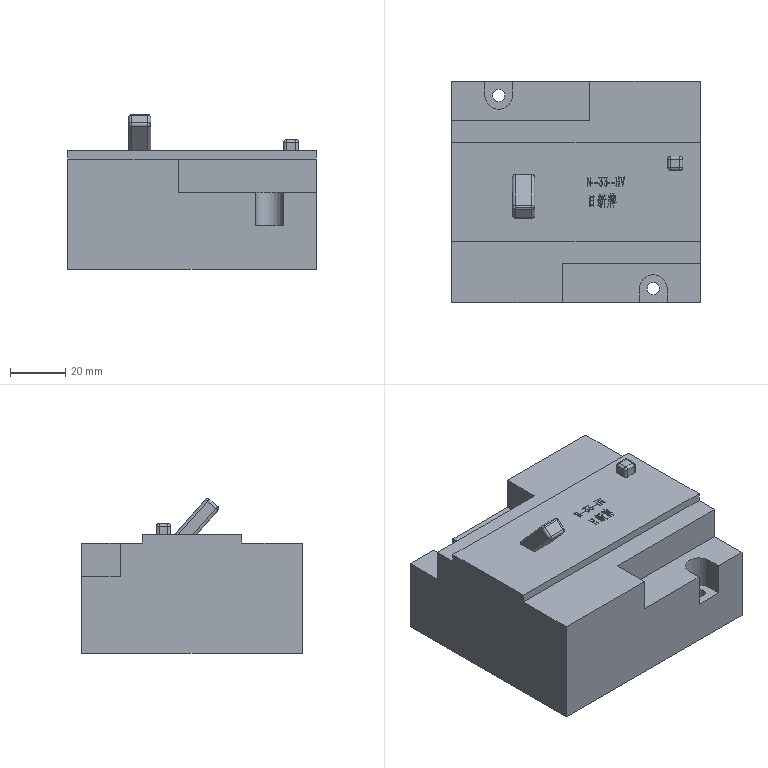Part | STEP file | QA-N-33-HV-1 | 1 solid | 514 faces | box 90 x 80 x 56.121 mm | volume 279078 mm3 | plane 344 | spline 138 | cylinder 23 | sphere 9 | commonest cylinder face diameters 2 x17 4.5 x4 10 x2